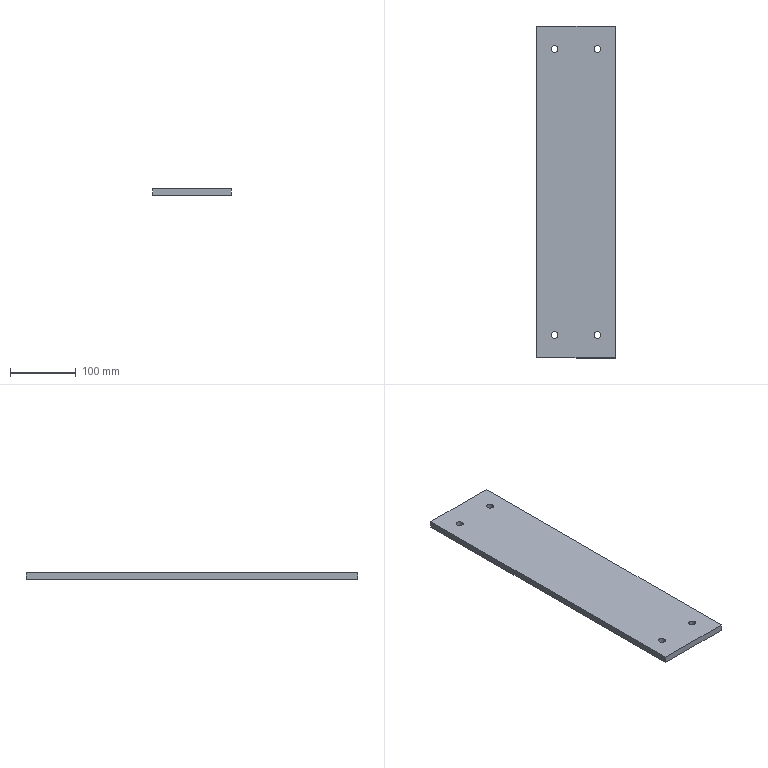Part | SolidWorks | features Extrusion 1, HoleWzd 1 | 1 solid | 14 faces | box 120 x 505 x 10 mm | volume 602731 mm3 | cylinder 8 | plane 6 | commonest cylinder face diameters 10.2 x8
STEP:
#1=CARTESIAN_POINT('',(-37.6,217.5,0.));
#2=VERTEX_POINT('',#1);
#3=CARTESIAN_POINT('',(-27.4,217.5,0.));
#4=VERTEX_POINT('',#3);
#5=CARTESIAN_POINT('',(-32.5,217.5,0.));
#6=DIRECTION('',(0.,0.,1.));
#7=DIRECTION('',(1.,0.,0.));
#8=AXIS2_PLACEMENT_3D('',#5,#6,#7);
#9=CIRCLE('',#8,5.1);
#10=EDGE_CURVE('',#2,#4,#9,.T.);
#11=ORIENTED_EDGE('',*,*,#10,.F.);
#12=CARTESIAN_POINT('',(-37.6,217.5,10.));
#13=VERTEX_POINT('',#12);
#14=CARTESIAN_POINT('',(-37.6,217.5,10.));
#15=DIRECTION('',(0.,0.,1.));
#16=VECTOR('',#15,1000.);
#17=LINE('',#14,#16);
#18=EDGE_CURVE('',#2,#13,#17,.T.);
#19=ORIENTED_EDGE('',*,*,#18,.T.);
#20=CARTESIAN_POINT('',(-27.4,217.5,10.));
#21=VERTEX_POINT('',#20);
#22=CARTESIAN_POINT('',(-32.5,217.5,10.));
#23=DIRECTION('',(0.,0.,1.));
#24=DIRECTION('',(1.,0.,0.));
#25=AXIS2_PLACEMENT_3D('',#22,#23,#24);
#26=CIRCLE('',#25,5.1);
#27=EDGE_CURVE('',#13,#21,#26,.T.);
#28=ORIENTED_EDGE('',*,*,#27,.T.);
#29=CARTESIAN_POINT('',(-27.4,217.5,10.));
#30=DIRECTION('',(0.,0.,1.));
#31=VECTOR('',#30,1000.);
#32=LINE('',#29,#31);
#33=EDGE_CURVE('',#4,#21,#32,.T.);
#34=ORIENTED_EDGE('',*,*,#33,.F.);
#35=EDGE_LOOP('',(#11,#19,#28,#34));
#36=FACE_OUTER_BOUND('',#35,.T.);
#37=CARTESIAN_POINT('',(-32.5,217.5,10.));
#38=DIRECTION('',(0.,0.,1.));
#39=DIRECTION('',(1.,0.,0.));
#40=AXIS2_PLACEMENT_3D('',#37,#38,#39);
#41=CYLINDRICAL_SURFACE('',#40,5.1);
#42=ADVANCED_FACE('',(#36),#41,.F.);
#43=CARTESIAN_POINT('',(27.4,217.5,0.));
#44=VERTEX_POINT('',#43);
#45=CARTESIAN_POINT('',(37.6,217.5,0.));
#46=VERTEX_POINT('',#45);
#47=CARTESIAN_POINT('',(32.5,217.5,0.));
#48=DIRECTION('',(0.,0.,1.));
#49=DIRECTION('',(1.,0.,0.));
#50=AXIS2_PLACEMENT_3D('',#47,#48,#49);
#51=CIRCLE('',#50,5.1);
#52=EDGE_CURVE('',#44,#46,#51,.T.);
#53=ORIENTED_EDGE('',*,*,#52,.F.);
#54=CARTESIAN_POINT('',(27.4,217.5,10.));
#55=VERTEX_POINT('',#54);
#56=CARTESIAN_POINT('',(27.4,217.5,10.));
#57=DIRECTION('',(0.,0.,1.));
#58=VECTOR('',#57,1000.);
#59=LINE('',#56,#58);
#60=EDGE_CURVE('',#44,#55,#59,.T.);
#61=ORIENTED_EDGE('',*,*,#60,.T.);
#62=CARTESIAN_POINT('',(37.6,217.5,10.));
#63=VERTEX_POINT('',#62);
#64=CARTESIAN_POINT('',(32.5,217.5,10.));
#65=DIRECTION('',(0.,0.,1.));
#66=DIRECTION('',(1.,0.,0.));
#67=AXIS2_PLACEMENT_3D('',#64,#65,#66);
#68=CIRCLE('',#67,5.1);
#69=EDGE_CURVE('',#55,#63,#68,.T.);
#70=ORIENTED_EDGE('',*,*,#69,.T.);
#71=CARTESIAN_POINT('',(37.6,217.5,10.));
#72=DIRECTION('',(0.,0.,1.));
#73=VECTOR('',#72,1000.);
#74=LINE('',#71,#73);
#75=EDGE_CURVE('',#46,#63,#74,.T.);
#76=ORIENTED_EDGE('',*,*,#75,.F.);
#77=EDGE_LOOP('',(#53,#61,#70,#76));
#78=FACE_OUTER_BOUND('',#77,.T.);
#79=CARTESIAN_POINT('',(32.5,217.5,10.));
#80=DIRECTION('',(0.,0.,1.));
#81=DIRECTION('',(1.,0.,0.));
#82=AXIS2_PLACEMENT_3D('',#79,#80,#81);
#83=CYLINDRICAL_SURFACE('',#82,5.1);
#84=ADVANCED_FACE('',(#78),#83,.F.);
#85=CARTESIAN_POINT('',(27.4,-217.5,0.));
#86=VERTEX_POINT('',#85);
#87=CARTESIAN_POINT('',(37.6,-217.5,0.));
#88=VERTEX_POINT('',#87);
#89=CARTESIAN_POINT('',(32.5,-217.5,0.));
#90=DIRECTION('',(0.,0.,1.));
#91=DIRECTION('',(1.,0.,0.));
#92=AXIS2_PLACEMENT_3D('',#89,#90,#91);
#93=CIRCLE('',#92,5.1);
#94=EDGE_CURVE('',#86,#88,#93,.T.);
#95=ORIENTED_EDGE('',*,*,#94,.F.);
#96=CARTESIAN_POINT('',(27.4,-217.5,10.));
#97=VERTEX_POINT('',#96);
#98=CARTESIAN_POINT('',(27.4,-217.5,10.));
#99=DIRECTION('',(0.,0.,1.));
#100=VECTOR('',#99,1000.);
#101=LINE('',#98,#100);
#102=EDGE_CURVE('',#86,#97,#101,.T.);
#103=ORIENTED_EDGE('',*,*,#102,.T.);
#104=CARTESIAN_POINT('',(37.6,-217.5,10.));
#105=VERTEX_POINT('',#104);
#106=CARTESIAN_POINT('',(32.5,-217.5,10.));
#107=DIRECTION('',(0.,0.,1.));
#108=DIRECTION('',(1.,0.,0.));
#109=AXIS2_PLACEMENT_3D('',#106,#107,#108);
#110=CIRCLE('',#109,5.1);
#111=EDGE_CURVE('',#97,#105,#110,.T.);
#112=ORIENTED_EDGE('',*,*,#111,.T.);
#113=CARTESIAN_POINT('',(37.6,-217.5,10.));
#114=DIRECTION('',(0.,0.,1.));
#115=VECTOR('',#114,1000.);
#116=LINE('',#113,#115);
#117=EDGE_CURVE('',#88,#105,#116,.T.);
#118=ORIENTED_EDGE('',*,*,#117,.F.);
#119=EDGE_LOOP('',(#95,#103,#112,#118));
#120=FACE_OUTER_BOUND('',#119,.T.);
#121=CARTESIAN_POINT('',(32.5,-217.5,10.));
#122=DIRECTION('',(0.,0.,1.));
#123=DIRECTION('',(1.,0.,0.));
#124=AXIS2_PLACEMENT_3D('',#121,#122,#123);
#125=CYLINDRICAL_SURFACE('',#124,5.1);
#126=ADVANCED_FACE('',(#120),#125,.F.);
#127=CARTESIAN_POINT('',(-37.6,-217.5,0.));
#128=VERTEX_POINT('',#127);
#129=CARTESIAN_POINT('',(-27.4,-217.5,0.));
#130=VERTEX_POINT('',#129);
#131=CARTESIAN_POINT('',(-32.5,-217.5,0.));
#132=DIRECTION('',(0.,0.,1.));
#133=DIRECTION('',(1.,0.,0.));
#134=AXIS2_PLACEMENT_3D('',#131,#132,#133);
#135=CIRCLE('',#134,5.1);
#136=EDGE_CURVE('',#128,#130,#135,.T.);
#137=ORIENTED_EDGE('',*,*,#136,.F.);
#138=CARTESIAN_POINT('',(-37.6,-217.5,10.));
#139=VERTEX_POINT('',#138);
#140=CARTESIAN_POINT('',(-37.6,-217.5,10.));
#141=DIRECTION('',(0.,0.,1.));
#142=VECTOR('',#141,1000.);
#143=LINE('',#140,#142);
#144=EDGE_CURVE('',#128,#139,#143,.T.);
#145=ORIENTED_EDGE('',*,*,#144,.T.);
#146=CARTESIAN_POINT('',(-27.4,-217.5,10.));
#147=VERTEX_POINT('',#146);
#148=CARTESIAN_POINT('',(-32.5,-217.5,10.));
#149=DIRECTION('',(0.,0.,1.));
#150=DIRECTION('',(1.,0.,0.));
#151=AXIS2_PLACEMENT_3D('',#148,#149,#150);
#152=CIRCLE('',#151,5.1);
#153=EDGE_CURVE('',#139,#147,#152,.T.);
#154=ORIENTED_EDGE('',*,*,#153,.T.);
#155=CARTESIAN_POINT('',(-27.4,-217.5,10.));
#156=DIRECTION('',(0.,0.,1.));
#157=VECTOR('',#156,1000.);
#158=LINE('',#155,#157);
#159=EDGE_CURVE('',#130,#147,#158,.T.);
#160=ORIENTED_EDGE('',*,*,#159,.F.);
#161=EDGE_LOOP('',(#137,#145,#154,#160));
#162=FACE_OUTER_BOUND('',#161,.T.);
#163=CARTESIAN_POINT('',(-32.5,-217.5,10.));
#164=DIRECTION('',(0.,0.,1.));
#165=DIRECTION('',(1.,0.,0.));
#166=AXIS2_PLACEMENT_3D('',#163,#164,#165);
#167=CYLINDRICAL_SURFACE('',#166,5.1);
#168=ADVANCED_FACE('',(#162),#167,.F.);
#169=CARTESIAN_POINT('',(60.,252.5,0.));
#170=VERTEX_POINT('',#169);
#171=CARTESIAN_POINT('',(-60.,252.5,0.));
#172=VERTEX_POINT('',#171);
#173=CARTESIAN_POINT('',(60.,252.5,0.));
#174=DIRECTION('',(-1.,0.,0.));
#175=VECTOR('',#174,1000.);
#176=LINE('',#173,#175);
#177=EDGE_CURVE('',#170,#172,#176,.T.);
#178=ORIENTED_EDGE('',*,*,#177,.T.);
#179=CARTESIAN_POINT('',(-60.,252.5,10.));
#180=VERTEX_POINT('',#179);
#181=CARTESIAN_POINT('',(-60.,252.5,10.));
#182=DIRECTION('',(0.,0.,-1.));
#183=VECTOR('',#182,1000.);
#184=LINE('',#181,#183);
#185=EDGE_CURVE('',#180,#172,#184,.T.);
#186=ORIENTED_EDGE('',*,*,#185,.F.);
#187=CARTESIAN_POINT('',(60.,252.5,10.));
#188=VERTEX_POINT('',#187);
#189=CARTESIAN_POINT('',(60.,252.5,10.));
#190=DIRECTION('',(-1.,0.,0.));
#191=VECTOR('',#190,1000.);
#192=LINE('',#189,#191);
#193=EDGE_CURVE('',#188,#180,#192,.T.);
#194=ORIENTED_EDGE('',*,*,#193,.F.);
#195=CARTESIAN_POINT('',(60.,252.5,10.));
#196=DIRECTION('',(0.,0.,-1.));
#197=VECTOR('',#196,1000.);
#198=LINE('',#195,#197);
#199=EDGE_CURVE('',#188,#170,#198,.T.);
#200=ORIENTED_EDGE('',*,*,#199,.T.);
#201=EDGE_LOOP('',(#178,#186,#194,#200));
#202=FACE_OUTER_BOUND('',#201,.T.);
#203=CARTESIAN_POINT('',(60.,252.5,10.));
#204=DIRECTION('',(0.,-1.,0.));
#205=DIRECTION('',(1.,0.,0.));
#206=AXIS2_PLACEMENT_3D('',#203,#204,#205);
#207=PLANE('',#206);
#208=ADVANCED_FACE('',(#202),#207,.F.);
#209=CARTESIAN_POINT('',(-60.,-252.5,0.));
#210=VERTEX_POINT('',#209);
#211=CARTESIAN_POINT('',(-60.,252.5,0.));
#212=DIRECTION('',(0.,-1.,0.));
#213=VECTOR('',#212,1000.);
#214=LINE('',#211,#213);
#215=EDGE_CURVE('',#172,#210,#214,.T.);
#216=ORIENTED_EDGE('',*,*,#215,.T.);
#217=CARTESIAN_POINT('',(-60.,-252.5,10.));
#218=VERTEX_POINT('',#217);
#219=CARTESIAN_POINT('',(-60.,-252.5,10.));
#220=DIRECTION('',(0.,0.,-1.));
#221=VECTOR('',#220,1000.);
#222=LINE('',#219,#221);
#223=EDGE_CURVE('',#218,#210,#222,.T.);
#224=ORIENTED_EDGE('',*,*,#223,.F.);
#225=CARTESIAN_POINT('',(-60.,252.5,10.));
#226=DIRECTION('',(0.,-1.,0.));
#227=VECTOR('',#226,1000.);
#228=LINE('',#225,#227);
#229=EDGE_CURVE('',#180,#218,#228,.T.);
#230=ORIENTED_EDGE('',*,*,#229,.F.);
#231=ORIENTED_EDGE('',*,*,#185,.T.);
#232=EDGE_LOOP('',(#216,#224,#230,#231));
#233=FACE_OUTER_BOUND('',#232,.T.);
#234=CARTESIAN_POINT('',(-60.,252.5,10.));
#235=DIRECTION('',(1.,0.,0.));
#236=DIRECTION('',(0.,1.,0.));
#237=AXIS2_PLACEMENT_3D('',#234,#235,#236);
#238=PLANE('',#237);
#239=ADVANCED_FACE('',(#233),#238,.F.);
#240=CARTESIAN_POINT('',(60.,-252.5,0.));
#241=VERTEX_POINT('',#240);
#242=CARTESIAN_POINT('',(60.,-252.5,0.));
#243=DIRECTION('',(-1.,0.,0.));
#244=VECTOR('',#243,1000.);
#245=LINE('',#242,#244);
#246=EDGE_CURVE('',#241,#210,#245,.T.);
#247=ORIENTED_EDGE('',*,*,#246,.F.);
#248=CARTESIAN_POINT('',(60.,-252.5,10.));
#249=VERTEX_POINT('',#248);
#250=CARTESIAN_POINT('',(60.,-252.5,10.));
#251=DIRECTION('',(0.,0.,-1.));
#252=VECTOR('',#251,1000.);
#253=LINE('',#250,#252);
#254=EDGE_CURVE('',#249,#241,#253,.T.);
#255=ORIENTED_EDGE('',*,*,#254,.F.);
#256=CARTESIAN_POINT('',(60.,-252.5,10.));
#257=DIRECTION('',(-1.,0.,0.));
#258=VECTOR('',#257,1000.);
#259=LINE('',#256,#258);
#260=EDGE_CURVE('',#249,#218,#259,.T.);
#261=ORIENTED_EDGE('',*,*,#260,.T.);
#262=ORIENTED_EDGE('',*,*,#223,.T.);
#263=EDGE_LOOP('',(#247,#255,#261,#262));
#264=FACE_OUTER_BOUND('',#263,.T.);
#265=CARTESIAN_POINT('',(60.,-252.5,10.));
#266=DIRECTION('',(0.,-1.,0.));
#267=DIRECTION('',(1.,0.,0.));
#268=AXIS2_PLACEMENT_3D('',#265,#266,#267);
#269=PLANE('',#268);
#270=ADVANCED_FACE('',(#264),#269,.T.);
#271=CARTESIAN_POINT('',(60.,252.5,0.));
#272=DIRECTION('',(0.,-1.,0.));
#273=VECTOR('',#272,1000.);
#274=LINE('',#271,#273);
#275=EDGE_CURVE('',#170,#241,#274,.T.);
#276=ORIENTED_EDGE('',*,*,#275,.F.);
#277=ORIENTED_EDGE('',*,*,#199,.F.);
#278=CARTESIAN_POINT('',(60.,252.5,10.));
#279=DIRECTION('',(0.,-1.,0.));
#280=VECTOR('',#279,1000.);
#281=LINE('',#278,#280);
#282=EDGE_CURVE('',#188,#249,#281,.T.);
#283=ORIENTED_EDGE('',*,*,#282,.T.);
#284=ORIENTED_EDGE('',*,*,#254,.T.);
#285=EDGE_LOOP('',(#276,#277,#283,#284));
#286=FACE_OUTER_BOUND('',#285,.T.);
#287=CARTESIAN_POINT('',(60.,252.5,10.));
#288=DIRECTION('',(1.,0.,0.));
#289=DIRECTION('',(0.,1.,0.));
#290=AXIS2_PLACEMENT_3D('',#287,#288,#289);
#291=PLANE('',#290);
#292=ADVANCED_FACE('',(#286),#291,.T.);
#293=CARTESIAN_POINT('',(-32.5,217.5,10.));
#294=DIRECTION('',(0.,0.,1.));
#295=DIRECTION('',(1.,0.,0.));
#296=AXIS2_PLACEMENT_3D('',#293,#294,#295);
#297=CIRCLE('',#296,5.1);
#298=EDGE_CURVE('',#21,#13,#297,.T.);
#299=ORIENTED_EDGE('',*,*,#298,.F.);
#300=ORIENTED_EDGE('',*,*,#27,.F.);
#301=EDGE_LOOP('',(#299,#300));
#302=FACE_BOUND('',#301,.T.);
#303=CARTESIAN_POINT('',(32.5,217.5,10.));
#304=DIRECTION('',(0.,0.,1.));
#305=DIRECTION('',(1.,0.,0.));
#306=AXIS2_PLACEMENT_3D('',#303,#304,#305);
#307=CIRCLE('',#306,5.1);
#308=EDGE_CURVE('',#63,#55,#307,.T.);
#309=ORIENTED_EDGE('',*,*,#308,.F.);
#310=ORIENTED_EDGE('',*,*,#69,.F.);
#311=EDGE_LOOP('',(#309,#310));
#312=FACE_BOUND('',#311,.T.);
#313=CARTESIAN_POINT('',(32.5,-217.5,10.));
#314=DIRECTION('',(0.,0.,1.));
#315=DIRECTION('',(1.,0.,0.));
#316=AXIS2_PLACEMENT_3D('',#313,#314,#315);
#317=CIRCLE('',#316,5.1);
#318=EDGE_CURVE('',#105,#97,#317,.T.);
#319=ORIENTED_EDGE('',*,*,#318,.F.);
#320=ORIENTED_EDGE('',*,*,#111,.F.);
#321=EDGE_LOOP('',(#319,#320));
#322=FACE_BOUND('',#321,.T.);
#323=CARTESIAN_POINT('',(-32.5,-217.5,10.));
#324=DIRECTION('',(0.,0.,1.));
#325=DIRECTION('',(1.,0.,0.));
#326=AXIS2_PLACEMENT_3D('',#323,#324,#325);
#327=CIRCLE('',#326,5.1);
#328=EDGE_CURVE('',#147,#139,#327,.T.);
#329=ORIENTED_EDGE('',*,*,#328,.F.);
#330=ORIENTED_EDGE('',*,*,#153,.F.);
#331=EDGE_LOOP('',(#329,#330));
#332=FACE_BOUND('',#331,.T.);
#333=ORIENTED_EDGE('',*,*,#193,.T.);
#334=ORIENTED_EDGE('',*,*,#229,.T.);
#335=ORIENTED_EDGE('',*,*,#260,.F.);
#336=ORIENTED_EDGE('',*,*,#282,.F.);
#337=EDGE_LOOP('',(#333,#334,#335,#336));
#338=FACE_OUTER_BOUND('',#337,.T.);
#339=CARTESIAN_POINT('',(0.,0.,10.));
#340=DIRECTION('',(0.,0.,1.));
#341=DIRECTION('',(1.,0.,0.));
#342=AXIS2_PLACEMENT_3D('',#339,#340,#341);
#343=PLANE('',#342);
#344=ADVANCED_FACE('',(#302,#312,#322,#332,#338),#343,.T.);
#345=CARTESIAN_POINT('',(-32.5,217.5,0.));
#346=DIRECTION('',(0.,0.,1.));
#347=DIRECTION('',(1.,0.,0.));
#348=AXIS2_PLACEMENT_3D('',#345,#346,#347);
#349=CIRCLE('',#348,5.1);
#350=EDGE_CURVE('',#4,#2,#349,.T.);
#351=ORIENTED_EDGE('',*,*,#350,.T.);
#352=ORIENTED_EDGE('',*,*,#10,.T.);
#353=EDGE_LOOP('',(#351,#352));
#354=FACE_BOUND('',#353,.T.);
#355=CARTESIAN_POINT('',(32.5,217.5,0.));
#356=DIRECTION('',(0.,0.,1.));
#357=DIRECTION('',(1.,0.,0.));
#358=AXIS2_PLACEMENT_3D('',#355,#356,#357);
#359=CIRCLE('',#358,5.1);
#360=EDGE_CURVE('',#46,#44,#359,.T.);
#361=ORIENTED_EDGE('',*,*,#360,.T.);
#362=ORIENTED_EDGE('',*,*,#52,.T.);
#363=EDGE_LOOP('',(#361,#362));
#364=FACE_BOUND('',#363,.T.);
#365=CARTESIAN_POINT('',(32.5,-217.5,0.));
#366=DIRECTION('',(0.,0.,1.));
#367=DIRECTION('',(1.,0.,0.));
#368=AXIS2_PLACEMENT_3D('',#365,#366,#367);
#369=CIRCLE('',#368,5.1);
#370=EDGE_CURVE('',#88,#86,#369,.T.);
#371=ORIENTED_EDGE('',*,*,#370,.T.);
#372=ORIENTED_EDGE('',*,*,#94,.T.);
#373=EDGE_LOOP('',(#371,#372));
#374=FACE_BOUND('',#373,.T.);
#375=CARTESIAN_POINT('',(-32.5,-217.5,0.));
#376=DIRECTION('',(0.,0.,1.));
#377=DIRECTION('',(1.,0.,0.));
#378=AXIS2_PLACEMENT_3D('',#375,#376,#377);
#379=CIRCLE('',#378,5.1);
#380=EDGE_CURVE('',#130,#128,#379,.T.);
#381=ORIENTED_EDGE('',*,*,#380,.T.);
#382=ORIENTED_EDGE('',*,*,#136,.T.);
#383=EDGE_LOOP('',(#381,#382));
#384=FACE_BOUND('',#383,.T.);
#385=ORIENTED_EDGE('',*,*,#177,.F.);
#386=ORIENTED_EDGE('',*,*,#275,.T.);
#387=ORIENTED_EDGE('',*,*,#246,.T.);
#388=ORIENTED_EDGE('',*,*,#215,.F.);
#389=EDGE_LOOP('',(#385,#386,#387,#388));
#390=FACE_OUTER_BOUND('',#389,.T.);
#391=CARTESIAN_POINT('',(0.,0.,0.));
#392=DIRECTION('',(0.,0.,1.));
#393=DIRECTION('',(1.,0.,0.));
#394=AXIS2_PLACEMENT_3D('',#391,#392,#393);
#395=PLANE('',#394);
#396=ADVANCED_FACE('',(#354,#364,#374,#384,#390),#395,.F.);
#397=ORIENTED_EDGE('',*,*,#144,.F.);
#398=ORIENTED_EDGE('',*,*,#380,.F.);
#399=ORIENTED_EDGE('',*,*,#159,.T.);
#400=ORIENTED_EDGE('',*,*,#328,.T.);
#401=EDGE_LOOP('',(#397,#398,#399,#400));
#402=FACE_OUTER_BOUND('',#401,.T.);
#403=CARTESIAN_POINT('',(-32.5,-217.5,10.));
#404=DIRECTION('',(0.,0.,1.));
#405=DIRECTION('',(1.,0.,0.));
#406=AXIS2_PLACEMENT_3D('',#403,#404,#405);
#407=CYLINDRICAL_SURFACE('',#406,5.1);
#408=ADVANCED_FACE('',(#402),#407,.F.);
#409=ORIENTED_EDGE('',*,*,#102,.F.);
#410=ORIENTED_EDGE('',*,*,#370,.F.);
#411=ORIENTED_EDGE('',*,*,#117,.T.);
#412=ORIENTED_EDGE('',*,*,#318,.T.);
#413=EDGE_LOOP('',(#409,#410,#411,#412));
#414=FACE_OUTER_BOUND('',#413,.T.);
#415=CARTESIAN_POINT('',(32.5,-217.5,10.));
#416=DIRECTION('',(0.,0.,1.));
#417=DIRECTION('',(1.,0.,0.));
#418=AXIS2_PLACEMENT_3D('',#415,#416,#417);
#419=CYLINDRICAL_SURFACE('',#418,5.1);
#420=ADVANCED_FACE('',(#414),#419,.F.);
#421=ORIENTED_EDGE('',*,*,#60,.F.);
#422=ORIENTED_EDGE('',*,*,#360,.F.);
#423=ORIENTED_EDGE('',*,*,#75,.T.);
#424=ORIENTED_EDGE('',*,*,#308,.T.);
#425=EDGE_LOOP('',(#421,#422,#423,#424));
#426=FACE_OUTER_BOUND('',#425,.T.);
#427=CARTESIAN_POINT('',(32.5,217.5,10.));
#428=DIRECTION('',(0.,0.,1.));
#429=DIRECTION('',(1.,0.,0.));
#430=AXIS2_PLACEMENT_3D('',#427,#428,#429);
#431=CYLINDRICAL_SURFACE('',#430,5.1);
#432=ADVANCED_FACE('',(#426),#431,.F.);
#433=ORIENTED_EDGE('',*,*,#18,.F.);
#434=ORIENTED_EDGE('',*,*,#350,.F.);
#435=ORIENTED_EDGE('',*,*,#33,.T.);
#436=ORIENTED_EDGE('',*,*,#298,.T.);
#437=EDGE_LOOP('',(#433,#434,#435,#436));
#438=FACE_OUTER_BOUND('',#437,.T.);
#439=CARTESIAN_POINT('',(-32.5,217.5,10.));
#440=DIRECTION('',(0.,0.,1.));
#441=DIRECTION('',(1.,0.,0.));
#442=AXIS2_PLACEMENT_3D('',#439,#440,#441);
#443=CYLINDRICAL_SURFACE('',#442,5.1);
#444=ADVANCED_FACE('',(#438),#443,.F.);
#445=CLOSED_SHELL('',(#42,#84,#126,#168,#208,#239,#270,#292,#344,#396,#408,#420,#432,#444));
#446=MANIFOLD_SOLID_BREP('',#445);
#447=CARTESIAN_POINT('',(0.,0.,0.));
#448=DIRECTION('',(0.,0.,1.));
#449=DIRECTION('',(1.,0.,0.));
#450=AXIS2_PLACEMENT_3D('',#447,#448,#449);
#451=(LENGTH_UNIT()NAMED_UNIT(*)SI_UNIT(.MILLI.,.METRE.));
#452=UNCERTAINTY_MEASURE_WITH_UNIT(LENGTH_MEASURE(0.00001),#451,'','');
#453=(NAMED_UNIT(*)PLANE_ANGLE_UNIT()SI_UNIT($,.RADIAN.));
#454=(NAMED_UNIT(*)SI_UNIT($,.STERADIAN.)SOLID_ANGLE_UNIT());
#455=(GEOMETRIC_REPRESENTATION_CONTEXT(3)GLOBAL_UNCERTAINTY_ASSIGNED_CONTEXT((#452))GLOBAL_UNIT_ASSIGNED_CONTEXT((#451,#453,#454))REPRESENTATION_CONTEXT('',''));
#456=ADVANCED_BREP_SHAPE_REPRESENTATION('',(#446,#450),#455);